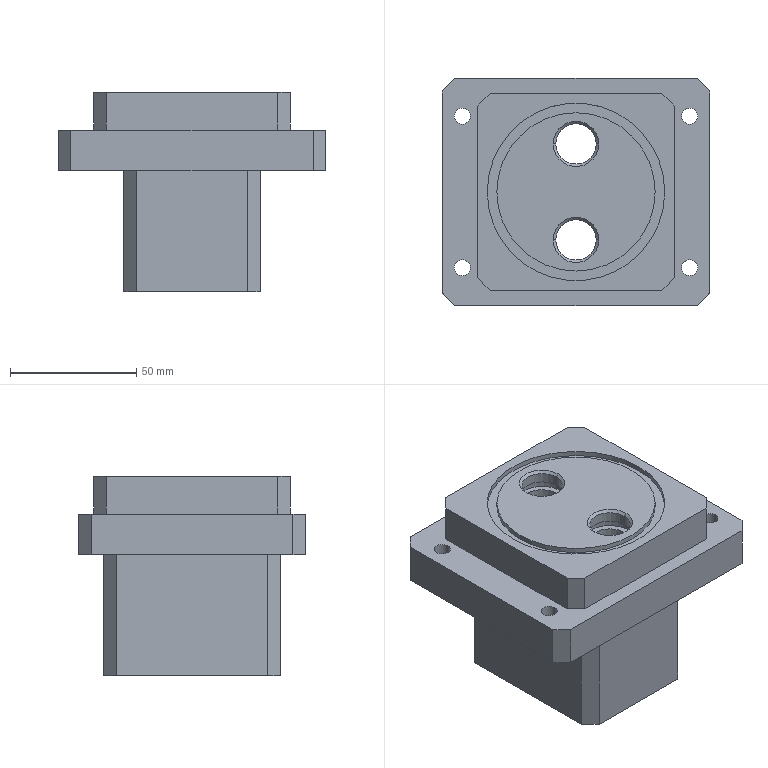Part | SolidWorks | features HoleWzd 4, ICE 4, Chamfer 2, Extrusion 1 | 1 solid | 100 faces | box 106 x 90 x 79 mm | volume 359467 mm3 | cylinder 44 | plane 40 | cone 16 | commonest cylinder face diameters 4.2 x8 6.4 x8 11 x8 16 x8 20.6 x4 22 x4